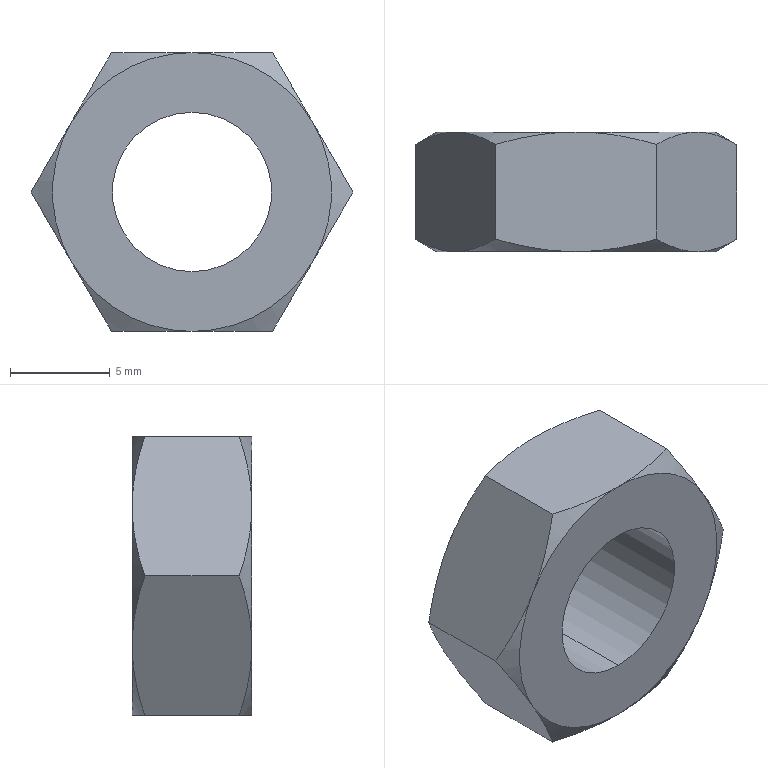Part | 1 solid | 22 faces | box 16.166 x 6 x 14 mm | volume 710.893 mm3 | cone 12 | plane 8 | cylinder 2 | commonest cylinder face diameters 8 x2
STEP:
#1=CARTESIAN_POINT('',(0.,6.,-4.));
#2=VERTEX_POINT('',#1);
#3=CARTESIAN_POINT('',(0.,6.,4.));
#4=VERTEX_POINT('',#3);
#5=CARTESIAN_POINT('',(0.,6.,0.));
#6=DIRECTION('',(0.,1.,0.));
#7=DIRECTION('',(0.,0.,1.));
#8=AXIS2_PLACEMENT_3D('',#5,#6,#7);
#9=CIRCLE('',#8,4.);
#10=EDGE_CURVE('',#2,#4,#9,.T.);
#11=ORIENTED_EDGE('',*,*,#10,.T.);
#12=CARTESIAN_POINT('',(0.,0.,4.));
#13=VERTEX_POINT('',#12);
#14=CARTESIAN_POINT('',(0.,6.,4.));
#15=DIRECTION('',(0.,-1.,0.));
#16=VECTOR('',#15,1000.);
#17=LINE('',#14,#16);
#18=EDGE_CURVE('',#4,#13,#17,.T.);
#19=ORIENTED_EDGE('',*,*,#18,.T.);
#20=CARTESIAN_POINT('',(0.,0.,-4.));
#21=VERTEX_POINT('',#20);
#22=CARTESIAN_POINT('',(0.,0.,0.));
#23=DIRECTION('',(0.,1.,0.));
#24=DIRECTION('',(0.,0.,1.));
#25=AXIS2_PLACEMENT_3D('',#22,#23,#24);
#26=CIRCLE('',#25,4.);
#27=EDGE_CURVE('',#21,#13,#26,.T.);
#28=ORIENTED_EDGE('',*,*,#27,.F.);
#29=CARTESIAN_POINT('',(0.,6.,-4.));
#30=DIRECTION('',(0.,-1.,0.));
#31=VECTOR('',#30,1000.);
#32=LINE('',#29,#31);
#33=EDGE_CURVE('',#2,#21,#32,.T.);
#34=ORIENTED_EDGE('',*,*,#33,.F.);
#35=EDGE_LOOP('',(#11,#19,#28,#34));
#36=FACE_OUTER_BOUND('',#35,.T.);
#37=CARTESIAN_POINT('',(0.,6.,0.));
#38=DIRECTION('',(0.,-1.,0.));
#39=DIRECTION('',(0.,0.,-1.));
#40=AXIS2_PLACEMENT_3D('',#37,#38,#39);
#41=CYLINDRICAL_SURFACE('',#40,4.);
#42=ADVANCED_FACE('',(#36),#41,.F.);
#43=CARTESIAN_POINT('',(8.083,0.6252,0.));
#44=VERTEX_POINT('',#43);
#45=CARTESIAN_POINT('',(6.062,0.,3.5));
#46=VERTEX_POINT('',#45);
#47=CARTESIAN_POINT('',(8.083,0.6252,0.));
#48=CARTESIAN_POINT('',(7.911,0.5258,0.2984));
#49=CARTESIAN_POINT('',(7.742,0.438,0.59));
#50=CARTESIAN_POINT('',(7.493,0.3238,1.021));
#51=CARTESIAN_POINT('',(7.411,0.2886,1.164));
#52=CARTESIAN_POINT('',(7.287,0.2402,1.378));
#53=CARTESIAN_POINT('',(7.226,0.2171,1.484));
#54=CARTESIAN_POINT('',(7.165,0.1957,1.59));
#55=CARTESIAN_POINT('',(7.124,0.1817,1.661));
#56=CARTESIAN_POINT('',(7.104,0.1752,1.695));
#57=CARTESIAN_POINT('',(6.998,0.1408,1.88));
#58=CARTESIAN_POINT('',(6.913,0.1166,2.026));
#59=CARTESIAN_POINT('',(6.786,0.08533,2.246));
#60=CARTESIAN_POINT('',(6.744,0.07574,2.319));
#61=CARTESIAN_POINT('',(6.66,0.05825,2.465));
#62=CARTESIAN_POINT('',(6.619,0.05048,2.536));
#63=CARTESIAN_POINT('',(6.403,0.01442,2.909));
#64=CARTESIAN_POINT('',(6.233,0.,3.203));
#65=CARTESIAN_POINT('',(6.062,0.,3.5));
#66=B_SPLINE_CURVE_WITH_KNOTS('',3,(#47,#48,#49,#50,#51,#52,#53,#54,#55,#56,#57,#58,#59,#60,#61,#62,#63,#64,#65),.UNSPECIFIED.,.F.,.F.,(4,2,2,1,2,2,2,2,2,4),(0.,0.25,0.375,0.4375,0.4687,0.5,0.625,0.6875,0.75,1.),.UNSPECIFIED.);
#67=EDGE_CURVE('',#44,#46,#66,.T.);
#68=ORIENTED_EDGE('',*,*,#67,.F.);
#69=CARTESIAN_POINT('',(8.083,5.375,0.));
#70=VERTEX_POINT('',#69);
#71=CARTESIAN_POINT('',(8.083,6.,0.));
#72=DIRECTION('',(0.,-1.,0.));
#73=VECTOR('',#72,1000.);
#74=LINE('',#71,#73);
#75=EDGE_CURVE('',#70,#44,#74,.T.);
#76=ORIENTED_EDGE('',*,*,#75,.F.);
#77=CARTESIAN_POINT('',(6.062,6.,3.5));
#78=VERTEX_POINT('',#77);
#79=CARTESIAN_POINT('',(6.062,6.,3.5));
#80=CARTESIAN_POINT('',(6.148,6.,3.351));
#81=CARTESIAN_POINT('',(6.233,5.996,3.203));
#82=CARTESIAN_POINT('',(6.362,5.986,2.981));
#83=CARTESIAN_POINT('',(6.405,5.981,2.907));
#84=CARTESIAN_POINT('',(6.49,5.97,2.758));
#85=CARTESIAN_POINT('',(6.534,5.964,2.683));
#86=CARTESIAN_POINT('',(6.661,5.942,2.463));
#87=CARTESIAN_POINT('',(6.745,5.925,2.317));
#88=CARTESIAN_POINT('',(6.872,5.894,2.098));
#89=CARTESIAN_POINT('',(6.935,5.877,1.988));
#90=CARTESIAN_POINT('',(6.999,5.858,1.877));
#91=CARTESIAN_POINT('',(7.042,5.845,1.804));
#92=CARTESIAN_POINT('',(7.064,5.838,1.765));
#93=CARTESIAN_POINT('',(7.411,5.726,1.164));
#94=CARTESIAN_POINT('',(7.739,5.573,0.5959));
#95=CARTESIAN_POINT('',(8.083,5.375,0.));
#96=B_SPLINE_CURVE_WITH_KNOTS('',3,(#79,#80,#81,#82,#83,#84,#85,#86,#87,#88,#89,#90,#91,#92,#93,#94,#95),.UNSPECIFIED.,.F.,.F.,(4,2,2,2,2,1,2,2,4),(0.,0.125,0.1875,0.25,0.375,0.4375,0.4687,0.5,1.),.UNSPECIFIED.);
#97=EDGE_CURVE('',#78,#70,#96,.T.);
#98=ORIENTED_EDGE('',*,*,#97,.F.);
#99=CARTESIAN_POINT('',(4.041,5.375,7.));
#100=VERTEX_POINT('',#99);
#101=CARTESIAN_POINT('',(4.041,5.375,7.));
#102=CARTESIAN_POINT('',(4.214,5.474,6.702));
#103=CARTESIAN_POINT('',(4.382,5.562,6.41));
#104=CARTESIAN_POINT('',(4.631,5.676,5.978));
#105=CARTESIAN_POINT('',(4.714,5.711,5.836));
#106=CARTESIAN_POINT('',(4.837,5.76,5.622));
#107=CARTESIAN_POINT('',(4.898,5.783,5.516));
#108=CARTESIAN_POINT('',(4.96,5.804,5.41));
#109=CARTESIAN_POINT('',(5.001,5.818,5.339));
#110=CARTESIAN_POINT('',(5.02,5.825,5.305));
#111=CARTESIAN_POINT('',(5.127,5.859,5.12));
#112=CARTESIAN_POINT('',(5.211,5.883,4.974));
#113=CARTESIAN_POINT('',(5.338,5.915,4.754));
#114=CARTESIAN_POINT('',(5.38,5.924,4.681));
#115=CARTESIAN_POINT('',(5.465,5.942,4.535));
#116=CARTESIAN_POINT('',(5.506,5.95,4.464));
#117=CARTESIAN_POINT('',(5.721,5.986,4.091));
#118=CARTESIAN_POINT('',(5.891,6.,3.797));
#119=CARTESIAN_POINT('',(6.062,6.,3.5));
#120=B_SPLINE_CURVE_WITH_KNOTS('',3,(#101,#102,#103,#104,#105,#106,#107,#108,#109,#110,#111,#112,#113,#114,#115,#116,#117,#118,#119),.UNSPECIFIED.,.F.,.F.,(4,2,2,1,2,2,2,2,2,4),(0.,0.25,0.375,0.4375,0.4688,0.5,0.625,0.6875,0.75,1.),.UNSPECIFIED.);
#121=EDGE_CURVE('',#100,#78,#120,.T.);
#122=ORIENTED_EDGE('',*,*,#121,.F.);
#123=CARTESIAN_POINT('',(4.041,0.6252,7.));
#124=VERTEX_POINT('',#123);
#125=CARTESIAN_POINT('',(4.041,6.,7.));
#126=DIRECTION('',(0.,-1.,0.));
#127=VECTOR('',#126,1000.);
#128=LINE('',#125,#127);
#129=EDGE_CURVE('',#100,#124,#128,.T.);
#130=ORIENTED_EDGE('',*,*,#129,.T.);
#131=CARTESIAN_POINT('',(6.062,0.,3.5));
#132=CARTESIAN_POINT('',(5.976,0.,3.649));
#133=CARTESIAN_POINT('',(5.891,0.003614,3.797));
#134=CARTESIAN_POINT('',(5.763,0.01446,4.019));
#135=CARTESIAN_POINT('',(5.72,0.01898,4.093));
#136=CARTESIAN_POINT('',(5.634,0.02982,4.242));
#137=CARTESIAN_POINT('',(5.59,0.03629,4.317));
#138=CARTESIAN_POINT('',(5.464,0.05753,4.537));
#139=CARTESIAN_POINT('',(5.379,0.07506,4.683));
#140=CARTESIAN_POINT('',(5.253,0.1064,4.902));
#141=CARTESIAN_POINT('',(5.189,0.1234,5.012));
#142=CARTESIAN_POINT('',(5.125,0.1422,5.123));
#143=CARTESIAN_POINT('',(5.083,0.1552,5.196));
#144=CARTESIAN_POINT('',(5.061,0.1622,5.235));
#145=CARTESIAN_POINT('',(4.714,0.2744,5.836));
#146=CARTESIAN_POINT('',(4.386,0.4266,6.404));
#147=CARTESIAN_POINT('',(4.041,0.6252,7.));
#148=B_SPLINE_CURVE_WITH_KNOTS('',3,(#131,#132,#133,#134,#135,#136,#137,#138,#139,#140,#141,#142,#143,#144,#145,#146,#147),.UNSPECIFIED.,.F.,.F.,(4,2,2,2,2,1,2,2,4),(0.,0.125,0.1875,0.25,0.375,0.4375,0.4687,0.5,1.),.UNSPECIFIED.);
#149=EDGE_CURVE('',#46,#124,#148,.T.);
#150=ORIENTED_EDGE('',*,*,#149,.F.);
#151=EDGE_LOOP('',(#68,#76,#98,#122,#130,#150));
#152=FACE_OUTER_BOUND('',#151,.T.);
#153=CARTESIAN_POINT('',(4.041,6.,7.));
#154=DIRECTION('',(-0.866,0.,-0.5));
#155=DIRECTION('',(-0.5,0.,0.866));
#156=AXIS2_PLACEMENT_3D('',#153,#154,#155);
#157=PLANE('',#156);
#158=ADVANCED_FACE('',(#152),#157,.F.);
#159=CARTESIAN_POINT('',(4.041,0.6252,-7.));
#160=VERTEX_POINT('',#159);
#161=CARTESIAN_POINT('',(6.062,0.,-3.5));
#162=VERTEX_POINT('',#161);
#163=CARTESIAN_POINT('',(4.041,0.6252,-7.));
#164=CARTESIAN_POINT('',(4.214,0.5258,-6.702));
#165=CARTESIAN_POINT('',(4.382,0.438,-6.41));
#166=CARTESIAN_POINT('',(4.631,0.3238,-5.978));
#167=CARTESIAN_POINT('',(4.714,0.2886,-5.836));
#168=CARTESIAN_POINT('',(4.837,0.2402,-5.622));
#169=CARTESIAN_POINT('',(4.898,0.2171,-5.516));
#170=CARTESIAN_POINT('',(4.96,0.1957,-5.41));
#171=CARTESIAN_POINT('',(5.001,0.1817,-5.339));
#172=CARTESIAN_POINT('',(5.02,0.1752,-5.305));
#173=CARTESIAN_POINT('',(5.127,0.1408,-5.12));
#174=CARTESIAN_POINT('',(5.211,0.1166,-4.974));
#175=CARTESIAN_POINT('',(5.338,0.08533,-4.754));
#176=CARTESIAN_POINT('',(5.38,0.07574,-4.681));
#177=CARTESIAN_POINT('',(5.465,0.05825,-4.535));
#178=CARTESIAN_POINT('',(5.506,0.05048,-4.464));
#179=CARTESIAN_POINT('',(5.721,0.01442,-4.091));
#180=CARTESIAN_POINT('',(5.891,0.,-3.797));
#181=CARTESIAN_POINT('',(6.062,0.,-3.5));
#182=B_SPLINE_CURVE_WITH_KNOTS('',3,(#163,#164,#165,#166,#167,#168,#169,#170,#171,#172,#173,#174,#175,#176,#177,#178,#179,#180,#181),.UNSPECIFIED.,.F.,.F.,(4,2,2,1,2,2,2,2,2,4),(0.,0.25,0.375,0.4375,0.4687,0.5,0.625,0.6875,0.75,1.),.UNSPECIFIED.);
#183=EDGE_CURVE('',#160,#162,#182,.T.);
#184=ORIENTED_EDGE('',*,*,#183,.F.);
#185=CARTESIAN_POINT('',(4.041,5.375,-7.));
#186=VERTEX_POINT('',#185);
#187=CARTESIAN_POINT('',(4.041,6.,-7.));
#188=DIRECTION('',(0.,-1.,0.));
#189=VECTOR('',#188,1000.);
#190=LINE('',#187,#189);
#191=EDGE_CURVE('',#186,#160,#190,.T.);
#192=ORIENTED_EDGE('',*,*,#191,.F.);
#193=CARTESIAN_POINT('',(6.062,6.,-3.5));
#194=VERTEX_POINT('',#193);
#195=CARTESIAN_POINT('',(6.062,6.,-3.5));
#196=CARTESIAN_POINT('',(5.976,6.,-3.649));
#197=CARTESIAN_POINT('',(5.891,5.996,-3.797));
#198=CARTESIAN_POINT('',(5.763,5.986,-4.019));
#199=CARTESIAN_POINT('',(5.72,5.981,-4.093));
#200=CARTESIAN_POINT('',(5.634,5.97,-4.242));
#201=CARTESIAN_POINT('',(5.59,5.964,-4.317));
#202=CARTESIAN_POINT('',(5.464,5.942,-4.537));
#203=CARTESIAN_POINT('',(5.379,5.925,-4.683));
#204=CARTESIAN_POINT('',(5.253,5.894,-4.902));
#205=CARTESIAN_POINT('',(5.189,5.877,-5.012));
#206=CARTESIAN_POINT('',(5.125,5.858,-5.123));
#207=CARTESIAN_POINT('',(5.083,5.845,-5.196));
#208=CARTESIAN_POINT('',(5.061,5.838,-5.235));
#209=CARTESIAN_POINT('',(4.714,5.726,-5.836));
#210=CARTESIAN_POINT('',(4.386,5.573,-6.404));
#211=CARTESIAN_POINT('',(4.041,5.375,-7.));
#212=B_SPLINE_CURVE_WITH_KNOTS('',3,(#195,#196,#197,#198,#199,#200,#201,#202,#203,#204,#205,#206,#207,#208,#209,#210,#211),.UNSPECIFIED.,.F.,.F.,(4,2,2,2,2,1,2,2,4),(0.,0.125,0.1875,0.25,0.375,0.4375,0.4687,0.5,1.),.UNSPECIFIED.);
#213=EDGE_CURVE('',#194,#186,#212,.T.);
#214=ORIENTED_EDGE('',*,*,#213,.F.);
#215=CARTESIAN_POINT('',(8.083,5.375,0.));
#216=CARTESIAN_POINT('',(7.911,5.474,-0.2984));
#217=CARTESIAN_POINT('',(7.742,5.562,-0.59));
#218=CARTESIAN_POINT('',(7.493,5.676,-1.021));
#219=CARTESIAN_POINT('',(7.411,5.711,-1.164));
#220=CARTESIAN_POINT('',(7.287,5.76,-1.378));
#221=CARTESIAN_POINT('',(7.226,5.783,-1.484));
#222=CARTESIAN_POINT('',(7.165,5.804,-1.59));
#223=CARTESIAN_POINT('',(7.124,5.818,-1.661));
#224=CARTESIAN_POINT('',(7.104,5.825,-1.695));
#225=CARTESIAN_POINT('',(6.998,5.859,-1.88));
#226=CARTESIAN_POINT('',(6.913,5.883,-2.026));
#227=CARTESIAN_POINT('',(6.786,5.915,-2.246));
#228=CARTESIAN_POINT('',(6.744,5.924,-2.319));
#229=CARTESIAN_POINT('',(6.66,5.942,-2.465));
#230=CARTESIAN_POINT('',(6.619,5.95,-2.536));
#231=CARTESIAN_POINT('',(6.403,5.986,-2.909));
#232=CARTESIAN_POINT('',(6.233,6.,-3.203));
#233=CARTESIAN_POINT('',(6.062,6.,-3.5));
#234=B_SPLINE_CURVE_WITH_KNOTS('',3,(#215,#216,#217,#218,#219,#220,#221,#222,#223,#224,#225,#226,#227,#228,#229,#230,#231,#232,#233),.UNSPECIFIED.,.F.,.F.,(4,2,2,1,2,2,2,2,2,4),(0.,0.25,0.375,0.4375,0.4688,0.5,0.625,0.6875,0.75,1.),.UNSPECIFIED.);
#235=EDGE_CURVE('',#70,#194,#234,.T.);
#236=ORIENTED_EDGE('',*,*,#235,.F.);
#237=ORIENTED_EDGE('',*,*,#75,.T.);
#238=CARTESIAN_POINT('',(6.062,0.,-3.5));
#239=CARTESIAN_POINT('',(6.148,0.,-3.351));
#240=CARTESIAN_POINT('',(6.233,0.003614,-3.203));
#241=CARTESIAN_POINT('',(6.362,0.01446,-2.981));
#242=CARTESIAN_POINT('',(6.405,0.01898,-2.907));
#243=CARTESIAN_POINT('',(6.49,0.02982,-2.758));
#244=CARTESIAN_POINT('',(6.534,0.03629,-2.683));
#245=CARTESIAN_POINT('',(6.661,0.05753,-2.463));
#246=CARTESIAN_POINT('',(6.745,0.07506,-2.317));
#247=CARTESIAN_POINT('',(6.872,0.1064,-2.098));
#248=CARTESIAN_POINT('',(6.935,0.1234,-1.988));
#249=CARTESIAN_POINT('',(6.999,0.1422,-1.877));
#250=CARTESIAN_POINT('',(7.042,0.1552,-1.804));
#251=CARTESIAN_POINT('',(7.064,0.1622,-1.765));
#252=CARTESIAN_POINT('',(7.411,0.2744,-1.164));
#253=CARTESIAN_POINT('',(7.739,0.4266,-0.5959));
#254=CARTESIAN_POINT('',(8.083,0.6252,0.));
#255=B_SPLINE_CURVE_WITH_KNOTS('',3,(#238,#239,#240,#241,#242,#243,#244,#245,#246,#247,#248,#249,#250,#251,#252,#253,#254),.UNSPECIFIED.,.F.,.F.,(4,2,2,2,2,1,2,2,4),(0.,0.125,0.1875,0.25,0.375,0.4375,0.4688,0.5,1.),.UNSPECIFIED.);
#256=EDGE_CURVE('',#162,#44,#255,.T.);
#257=ORIENTED_EDGE('',*,*,#256,.F.);
#258=EDGE_LOOP('',(#184,#192,#214,#236,#237,#257));
#259=FACE_OUTER_BOUND('',#258,.T.);
#260=CARTESIAN_POINT('',(8.083,6.,0.));
#261=DIRECTION('',(-0.866,0.,0.5));
#262=DIRECTION('',(0.,1.,0.));
#263=AXIS2_PLACEMENT_3D('',#260,#261,#262);
#264=PLANE('',#263);
#265=ADVANCED_FACE('',(#259),#264,.F.);
#266=CARTESIAN_POINT('',(-4.041,0.6252,-7.));
#267=VERTEX_POINT('',#266);
#268=CARTESIAN_POINT('',(0.,0.,-7.));
#269=VERTEX_POINT('',#268);
#270=CARTESIAN_POINT('',(-4.041,0.6252,-7.));
#271=CARTESIAN_POINT('',(-3.696,0.5255,-7.));
#272=CARTESIAN_POINT('',(-3.358,0.4375,-7.));
#273=CARTESIAN_POINT('',(-2.859,0.3231,-7.));
#274=CARTESIAN_POINT('',(-2.694,0.2879,-7.));
#275=CARTESIAN_POINT('',(-2.447,0.2395,-7.));
#276=CARTESIAN_POINT('',(-2.323,0.2164,-7.));
#277=CARTESIAN_POINT('',(-2.2,0.1949,-7.));
#278=CARTESIAN_POINT('',(-2.118,0.1809,-7.));
#279=CARTESIAN_POINT('',(-2.079,0.1744,-7.));
#280=CARTESIAN_POINT('',(-1.866,0.1401,-7.));
#281=CARTESIAN_POINT('',(-1.697,0.1159,-7.));
#282=CARTESIAN_POINT('',(-1.443,0.08477,-7.));
#283=CARTESIAN_POINT('',(-1.359,0.07522,-7.));
#284=CARTESIAN_POINT('',(-1.191,0.05779,-7.));
#285=CARTESIAN_POINT('',(-1.108,0.05002,-7.));
#286=CARTESIAN_POINT('',(-0.6791,0.01429,-7.));
#287=CARTESIAN_POINT('',(-0.3408,0.,-7.));
#288=CARTESIAN_POINT('',(0.,0.,-7.));
#289=B_SPLINE_CURVE_WITH_KNOTS('',3,(#270,#271,#272,#273,#274,#275,#276,#277,#278,#279,#280,#281,#282,#283,#284,#285,#286,#287,#288),.UNSPECIFIED.,.F.,.F.,(4,2,2,1,2,2,2,2,2,4),(0.,0.25,0.375,0.4375,0.4687,0.5,0.625,0.6875,0.75,1.),.UNSPECIFIED.);
#290=EDGE_CURVE('',#267,#269,#289,.T.);
#291=ORIENTED_EDGE('',*,*,#290,.F.);
#292=CARTESIAN_POINT('',(-4.041,5.375,-7.));
#293=VERTEX_POINT('',#292);
#294=CARTESIAN_POINT('',(-4.041,6.,-7.));
#295=DIRECTION('',(0.,-1.,0.));
#296=VECTOR('',#295,1000.);
#297=LINE('',#294,#296);
#298=EDGE_CURVE('',#293,#267,#297,.T.);
#299=ORIENTED_EDGE('',*,*,#298,.F.);
#300=CARTESIAN_POINT('',(0.,6.,-7.));
#301=VERTEX_POINT('',#300);
#302=CARTESIAN_POINT('',(0.,6.,-7.));
#303=CARTESIAN_POINT('',(-0.1704,6.,-7.));
#304=CARTESIAN_POINT('',(-0.3402,5.996,-7.));
#305=CARTESIAN_POINT('',(-0.5952,5.986,-7.));
#306=CARTESIAN_POINT('',(-0.6803,5.981,-7.));
#307=CARTESIAN_POINT('',(-0.8507,5.971,-7.));
#308=CARTESIAN_POINT('',(-0.9375,5.964,-7.));
#309=CARTESIAN_POINT('',(-1.191,5.943,-7.));
#310=CARTESIAN_POINT('',(-1.359,5.926,-7.));
#311=CARTESIAN_POINT('',(-1.612,5.894,-7.));
#312=CARTESIAN_POINT('',(-1.739,5.878,-7.));
#313=CARTESIAN_POINT('',(-1.866,5.859,-7.));
#314=CARTESIAN_POINT('',(-1.951,5.846,-7.));
#315=CARTESIAN_POINT('',(-1.995,5.839,-7.));
#316=CARTESIAN_POINT('',(-2.692,5.727,-7.));
#317=CARTESIAN_POINT('',(-3.351,5.574,-7.));
#318=CARTESIAN_POINT('',(-4.041,5.375,-7.));
#319=B_SPLINE_CURVE_WITH_KNOTS('',3,(#302,#303,#304,#305,#306,#307,#308,#309,#310,#311,#312,#313,#314,#315,#316,#317,#318),.UNSPECIFIED.,.F.,.F.,(4,2,2,2,2,1,2,2,4),(0.,0.125,0.1875,0.25,0.375,0.4375,0.4687,0.5,1.),.UNSPECIFIED.);
#320=EDGE_CURVE('',#301,#293,#319,.T.);
#321=ORIENTED_EDGE('',*,*,#320,.F.);
#322=CARTESIAN_POINT('',(4.041,5.375,-7.));
#323=CARTESIAN_POINT('',(3.699,5.474,-7.));
#324=CARTESIAN_POINT('',(3.364,5.561,-7.));
#325=CARTESIAN_POINT('',(2.868,5.675,-7.));
#326=CARTESIAN_POINT('',(2.704,5.71,-7.));
#327=CARTESIAN_POINT('',(2.459,5.758,-7.));
#328=CARTESIAN_POINT('',(2.336,5.781,-7.));
#329=CARTESIAN_POINT('',(2.214,5.803,-7.));
#330=CARTESIAN_POINT('',(2.133,5.817,-7.));
#331=CARTESIAN_POINT('',(2.094,5.823,-7.));
#332=CARTESIAN_POINT('',(1.88,5.858,-7.));
#333=CARTESIAN_POINT('',(1.71,5.882,-7.));
#334=CARTESIAN_POINT('',(1.455,5.914,-7.));
#335=CARTESIAN_POINT('',(1.37,5.924,-7.));
#336=CARTESIAN_POINT('',(1.2,5.941,-7.));
#337=CARTESIAN_POINT('',(1.116,5.949,-7.));
#338=CARTESIAN_POINT('',(0.6836,5.985,-7.));
#339=CARTESIAN_POINT('',(0.3428,6.,-7.));
#340=CARTESIAN_POINT('',(0.,6.,-7.));
#341=B_SPLINE_CURVE_WITH_KNOTS('',3,(#322,#323,#324,#325,#326,#327,#328,#329,#330,#331,#332,#333,#334,#335,#336,#337,#338,#339,#340),.UNSPECIFIED.,.F.,.F.,(4,2,2,1,2,2,2,2,2,4),(0.,0.25,0.375,0.4375,0.4688,0.5,0.625,0.6875,0.75,1.),.UNSPECIFIED.);
#342=EDGE_CURVE('',#186,#301,#341,.T.);
#343=ORIENTED_EDGE('',*,*,#342,.F.);
#344=ORIENTED_EDGE('',*,*,#191,.T.);
#345=CARTESIAN_POINT('',(0.,0.,-7.));
#346=CARTESIAN_POINT('',(0.1714,0.,-7.));
#347=CARTESIAN_POINT('',(0.3423,0.003632,-7.));
#348=CARTESIAN_POINT('',(0.5992,0.01453,-7.));
#349=CARTESIAN_POINT('',(0.685,0.01907,-7.));
#350=CARTESIAN_POINT('',(0.8569,0.02997,-7.));
#351=CARTESIAN_POINT('',(0.9444,0.03644,-7.));
#352=CARTESIAN_POINT('',(1.2,0.05789,-7.));
#353=CARTESIAN_POINT('',(1.37,0.07557,-7.));
#354=CARTESIAN_POINT('',(1.625,0.1072,-7.));
#355=CARTESIAN_POINT('',(1.752,0.1242,-7.));
#356=CARTESIAN_POINT('',(1.88,0.1432,-7.));
#357=CARTESIAN_POINT('',(1.966,0.1563,-7.));
#358=CARTESIAN_POINT('',(2.011,0.1634,-7.));
#359=CARTESIAN_POINT('',(2.702,0.2756,-7.));
#360=CARTESIAN_POINT('',(3.356,0.4273,-7.));
#361=CARTESIAN_POINT('',(4.041,0.6252,-7.));
#362=B_SPLINE_CURVE_WITH_KNOTS('',3,(#345,#346,#347,#348,#349,#350,#351,#352,#353,#354,#355,#356,#357,#358,#359,#360,#361),.UNSPECIFIED.,.F.,.F.,(4,2,2,2,2,1,2,2,4),(0.,0.125,0.1875,0.25,0.375,0.4375,0.4687,0.5,1.),.UNSPECIFIED.);
#363=EDGE_CURVE('',#269,#160,#362,.T.);
#364=ORIENTED_EDGE('',*,*,#363,.F.);
#365=EDGE_LOOP('',(#291,#299,#321,#343,#344,#364));
#366=FACE_OUTER_BOUND('',#365,.T.);
#367=CARTESIAN_POINT('',(4.041,6.,-7.));
#368=DIRECTION('',(0.,0.,1.));
#369=DIRECTION('',(1.,0.,0.));
#370=AXIS2_PLACEMENT_3D('',#367,#368,#369);
#371=PLANE('',#370);
#372=ADVANCED_FACE('',(#366),#371,.F.);
#373=CARTESIAN_POINT('',(-8.083,0.6252,0.));
#374=VERTEX_POINT('',#373);
#375=CARTESIAN_POINT('',(-6.062,0.,-3.5));
#376=VERTEX_POINT('',#375);
#377=CARTESIAN_POINT('',(-8.083,0.6252,0.));
#378=CARTESIAN_POINT('',(-7.911,0.5258,-0.2984));
#379=CARTESIAN_POINT('',(-7.742,0.438,-0.59));
#380=CARTESIAN_POINT('',(-7.493,0.3238,-1.021));
#381=CARTESIAN_POINT('',(-7.411,0.2886,-1.164));
#382=CARTESIAN_POINT('',(-7.287,0.2402,-1.378));
#383=CARTESIAN_POINT('',(-7.226,0.2171,-1.484));
#384=CARTESIAN_POINT('',(-7.165,0.1957,-1.59));
#385=CARTESIAN_POINT('',(-7.124,0.1817,-1.661));
#386=CARTESIAN_POINT('',(-7.104,0.1752,-1.695));
#387=CARTESIAN_POINT('',(-6.998,0.1408,-1.88));
#388=CARTESIAN_POINT('',(-6.913,0.1166,-2.026));
#389=CARTESIAN_POINT('',(-6.786,0.08533,-2.246));
#390=CARTESIAN_POINT('',(-6.744,0.07574,-2.319));
#391=CARTESIAN_POINT('',(-6.66,0.05825,-2.465));
#392=CARTESIAN_POINT('',(-6.619,0.05048,-2.536));
#393=CARTESIAN_POINT('',(-6.403,0.01442,-2.909));
#394=CARTESIAN_POINT('',(-6.233,0.,-3.203));
#395=CARTESIAN_POINT('',(-6.062,0.,-3.5));
#396=B_SPLINE_CURVE_WITH_KNOTS('',3,(#377,#378,#379,#380,#381,#382,#383,#384,#385,#386,#387,#388,#389,#390,#391,#392,#393,#394,#395),.UNSPECIFIED.,.F.,.F.,(4,2,2,1,2,2,2,2,2,4),(0.,0.25,0.375,0.4375,0.4687,0.5,0.625,0.6875,0.75,1.),.UNSPECIFIED.);
#397=EDGE_CURVE('',#374,#376,#396,.T.);
#398=ORIENTED_EDGE('',*,*,#397,.F.);
#399=CARTESIAN_POINT('',(-8.083,5.375,0.));
#400=VERTEX_POINT('',#399);
#401=CARTESIAN_POINT('',(-8.083,6.,0.));
#402=DIRECTION('',(0.,-1.,0.));
#403=VECTOR('',#402,1000.);
#404=LINE('',#401,#403);
#405=EDGE_CURVE('',#400,#374,#404,.T.);
#406=ORIENTED_EDGE('',*,*,#405,.F.);
#407=CARTESIAN_POINT('',(-6.062,6.,-3.5));
#408=VERTEX_POINT('',#407);
#409=CARTESIAN_POINT('',(-6.062,6.,-3.5));
#410=CARTESIAN_POINT('',(-6.148,6.,-3.351));
#411=CARTESIAN_POINT('',(-6.233,5.996,-3.203));
#412=CARTESIAN_POINT('',(-6.362,5.986,-2.981));
#413=CARTESIAN_POINT('',(-6.405,5.981,-2.907));
#414=CARTESIAN_POINT('',(-6.49,5.97,-2.758));
#415=CARTESIAN_POINT('',(-6.534,5.964,-2.683));
#416=CARTESIAN_POINT('',(-6.661,5.942,-2.463));
#417=CARTESIAN_POINT('',(-6.745,5.925,-2.317));
#418=CARTESIAN_POINT('',(-6.872,5.894,-2.098));
#419=CARTESIAN_POINT('',(-6.935,5.877,-1.988));
#420=CARTESIAN_POINT('',(-6.999,5.858,-1.877));
#421=CARTESIAN_POINT('',(-7.042,5.845,-1.804));
#422=CARTESIAN_POINT('',(-7.064,5.838,-1.765));
#423=CARTESIAN_POINT('',(-7.411,5.726,-1.164));
#424=CARTESIAN_POINT('',(-7.739,5.573,-0.5959));
#425=CARTESIAN_POINT('',(-8.083,5.375,0.));
#426=B_SPLINE_CURVE_WITH_KNOTS('',3,(#409,#410,#411,#412,#413,#414,#415,#416,#417,#418,#419,#420,#421,#422,#423,#424,#425),.UNSPECIFIED.,.F.,.F.,(4,2,2,2,2,1,2,2,4),(0.,0.125,0.1875,0.25,0.375,0.4375,0.4687,0.5,1.),.UNSPECIFIED.);
#427=EDGE_CURVE('',#408,#400,#426,.T.);
#428=ORIENTED_EDGE('',*,*,#427,.F.);
#429=CARTESIAN_POINT('',(-4.041,5.375,-7.));
#430=CARTESIAN_POINT('',(-4.214,5.474,-6.702));
#431=CARTESIAN_POINT('',(-4.382,5.562,-6.41));
#432=CARTESIAN_POINT('',(-4.631,5.676,-5.978));
#433=CARTESIAN_POINT('',(-4.714,5.711,-5.836));
#434=CARTESIAN_POINT('',(-4.837,5.76,-5.622));
#435=CARTESIAN_POINT('',(-4.898,5.783,-5.516));
#436=CARTESIAN_POINT('',(-4.96,5.804,-5.41));
#437=CARTESIAN_POINT('',(-5.001,5.818,-5.339));
#438=CARTESIAN_POINT('',(-5.02,5.825,-5.305));
#439=CARTESIAN_POINT('',(-5.127,5.859,-5.12));
#440=CARTESIAN_POINT('',(-5.211,5.883,-4.974));
#441=CARTESIAN_POINT('',(-5.338,5.915,-4.754));
#442=CARTESIAN_POINT('',(-5.38,5.924,-4.681));
#443=CARTESIAN_POINT('',(-5.465,5.942,-4.535));
#444=CARTESIAN_POINT('',(-5.506,5.95,-4.464));
#445=CARTESIAN_POINT('',(-5.721,5.986,-4.091));
#446=CARTESIAN_POINT('',(-5.891,6.,-3.797));
#447=CARTESIAN_POINT('',(-6.062,6.,-3.5));
#448=B_SPLINE_CURVE_WITH_KNOTS('',3,(#429,#430,#431,#432,#433,#434,#435,#436,#437,#438,#439,#440,#441,#442,#443,#444,#445,#446,#447),.UNSPECIFIED.,.F.,.F.,(4,2,2,1,2,2,2,2,2,4),(0.,0.25,0.375,0.4375,0.4688,0.5,0.625,0.6875,0.75,1.),.UNSPECIFIED.);
#449=EDGE_CURVE('',#293,#408,#448,.T.);
#450=ORIENTED_EDGE('',*,*,#449,.F.);
#451=ORIENTED_EDGE('',*,*,#298,.T.);
#452=CARTESIAN_POINT('',(-6.062,0.,-3.5));
#453=CARTESIAN_POINT('',(-5.976,0.,-3.649));
#454=CARTESIAN_POINT('',(-5.891,0.003614,-3.797));
#455=CARTESIAN_POINT('',(-5.763,0.01446,-4.019));
#456=CARTESIAN_POINT('',(-5.72,0.01898,-4.093));
#457=CARTESIAN_POINT('',(-5.634,0.02982,-4.242));
#458=CARTESIAN_POINT('',(-5.59,0.03629,-4.317));
#459=CARTESIAN_POINT('',(-5.464,0.05753,-4.537));
#460=CARTESIAN_POINT('',(-5.379,0.07506,-4.683));
#461=CARTESIAN_POINT('',(-5.253,0.1064,-4.902));
#462=CARTESIAN_POINT('',(-5.189,0.1234,-5.012));
#463=CARTESIAN_POINT('',(-5.125,0.1422,-5.123));
#464=CARTESIAN_POINT('',(-5.083,0.1552,-5.196));
#465=CARTESIAN_POINT('',(-5.061,0.1622,-5.235));
#466=CARTESIAN_POINT('',(-4.714,0.2744,-5.836));
#467=CARTESIAN_POINT('',(-4.386,0.4266,-6.404));
#468=CARTESIAN_POINT('',(-4.041,0.6252,-7.));
#469=B_SPLINE_CURVE_WITH_KNOTS('',3,(#452,#453,#454,#455,#456,#457,#458,#459,#460,#461,#462,#463,#464,#465,#466,#467,#468),.UNSPECIFIED.,.F.,.F.,(4,2,2,2,2,1,2,2,4),(0.,0.125,0.1875,0.25,0.375,0.4375,0.4687,0.5,1.),.UNSPECIFIED.);
#470=EDGE_CURVE('',#376,#267,#469,.T.);
#471=ORIENTED_EDGE('',*,*,#470,.F.);
#472=EDGE_LOOP('',(#398,#406,#428,#450,#451,#471));
#473=FACE_OUTER_BOUND('',#472,.T.);
#474=CARTESIAN_POINT('',(-4.041,6.,-7.));
#475=DIRECTION('',(0.866,0.,0.5));
#476=DIRECTION('',(0.,-1.,0.));
#477=AXIS2_PLACEMENT_3D('',#474,#475,#476);
#478=PLANE('',#477);
#479=ADVANCED_FACE('',(#473),#478,.F.);
#480=CARTESIAN_POINT('',(-4.041,0.6252,7.));
#481=VERTEX_POINT('',#480);
#482=CARTESIAN_POINT('',(-6.062,0.,3.5));
#483=VERTEX_POINT('',#482);
#484=CARTESIAN_POINT('',(-4.041,0.6252,7.));
#485=CARTESIAN_POINT('',(-4.214,0.5258,6.702));
#486=CARTESIAN_POINT('',(-4.382,0.438,6.41));
#487=CARTESIAN_POINT('',(-4.631,0.3238,5.978));
#488=CARTESIAN_POINT('',(-4.714,0.2886,5.836));
#489=CARTESIAN_POINT('',(-4.837,0.2402,5.622));
#490=CARTESIAN_POINT('',(-4.898,0.2171,5.516));
#491=CARTESIAN_POINT('',(-4.96,0.1957,5.41));
#492=CARTESIAN_POINT('',(-5.001,0.1817,5.339));
#493=CARTESIAN_POINT('',(-5.02,0.1752,5.305));
#494=CARTESIAN_POINT('',(-5.127,0.1408,5.12));
#495=CARTESIAN_POINT('',(-5.211,0.1166,4.974));
#496=CARTESIAN_POINT('',(-5.338,0.08533,4.754));
#497=CARTESIAN_POINT('',(-5.38,0.07574,4.681));
#498=CARTESIAN_POINT('',(-5.465,0.05825,4.535));
#499=CARTESIAN_POINT('',(-5.506,0.05048,4.464));
#500=CARTESIAN_POINT('',(-5.721,0.01442,4.091));
#501=CARTESIAN_POINT('',(-5.891,0.,3.797));
#502=CARTESIAN_POINT('',(-6.062,0.,3.5));
#503=B_SPLINE_CURVE_WITH_KNOTS('',3,(#484,#485,#486,#487,#488,#489,#490,#491,#492,#493,#494,#495,#496,#497,#498,#499,#500,#501,#502),.UNSPECIFIED.,.F.,.F.,(4,2,2,1,2,2,2,2,2,4),(0.,0.25,0.375,0.4375,0.4687,0.5,0.625,0.6875,0.75,1.),.UNSPECIFIED.);
#504=EDGE_CURVE('',#481,#483,#503,.T.);
#505=ORIENTED_EDGE('',*,*,#504,.F.);
#506=CARTESIAN_POINT('',(-4.041,5.375,7.));
#507=VERTEX_POINT('',#506);
#508=CARTESIAN_POINT('',(-4.041,6.,7.));
#509=DIRECTION('',(0.,-1.,0.));
#510=VECTOR('',#509,1000.);
#511=LINE('',#508,#510);
#512=EDGE_CURVE('',#507,#481,#511,.T.);
#513=ORIENTED_EDGE('',*,*,#512,.F.);
#514=CARTESIAN_POINT('',(-6.062,6.,3.5));
#515=VERTEX_POINT('',#514);
#516=CARTESIAN_POINT('',(-6.062,6.,3.5));
#517=CARTESIAN_POINT('',(-5.976,6.,3.649));
#518=CARTESIAN_POINT('',(-5.891,5.996,3.797));
#519=CARTESIAN_POINT('',(-5.763,5.986,4.019));
#520=CARTESIAN_POINT('',(-5.72,5.981,4.093));
#521=CARTESIAN_POINT('',(-5.634,5.97,4.242));
#522=CARTESIAN_POINT('',(-5.59,5.964,4.317));
#523=CARTESIAN_POINT('',(-5.464,5.942,4.537));
#524=CARTESIAN_POINT('',(-5.379,5.925,4.683));
#525=CARTESIAN_POINT('',(-5.253,5.894,4.902));
#526=CARTESIAN_POINT('',(-5.189,5.877,5.012));
#527=CARTESIAN_POINT('',(-5.125,5.858,5.123));
#528=CARTESIAN_POINT('',(-5.083,5.845,5.196));
#529=CARTESIAN_POINT('',(-5.061,5.838,5.235));
#530=CARTESIAN_POINT('',(-4.714,5.726,5.836));
#531=CARTESIAN_POINT('',(-4.386,5.573,6.404));
#532=CARTESIAN_POINT('',(-4.041,5.375,7.));
#533=B_SPLINE_CURVE_WITH_KNOTS('',3,(#516,#517,#518,#519,#520,#521,#522,#523,#524,#525,#526,#527,#528,#529,#530,#531,#532),.UNSPECIFIED.,.F.,.F.,(4,2,2,2,2,1,2,2,4),(0.,0.125,0.1875,0.25,0.375,0.4375,0.4687,0.5,1.),.UNSPECIFIED.);
#534=EDGE_CURVE('',#515,#507,#533,.T.);
#535=ORIENTED_EDGE('',*,*,#534,.F.);
#536=CARTESIAN_POINT('',(-8.083,5.375,0.));
#537=CARTESIAN_POINT('',(-7.911,5.474,0.2984));
#538=CARTESIAN_POINT('',(-7.742,5.562,0.59));
#539=CARTESIAN_POINT('',(-7.493,5.676,1.021));
#540=CARTESIAN_POINT('',(-7.411,5.711,1.164));
#541=CARTESIAN_POINT('',(-7.287,5.76,1.378));
#542=CARTESIAN_POINT('',(-7.226,5.783,1.484));
#543=CARTESIAN_POINT('',(-7.165,5.804,1.59));
#544=CARTESIAN_POINT('',(-7.124,5.818,1.661));
#545=CARTESIAN_POINT('',(-7.104,5.825,1.695));
#546=CARTESIAN_POINT('',(-6.998,5.859,1.88));
#547=CARTESIAN_POINT('',(-6.913,5.883,2.026));
#548=CARTESIAN_POINT('',(-6.786,5.915,2.246));
#549=CARTESIAN_POINT('',(-6.744,5.924,2.319));
#550=CARTESIAN_POINT('',(-6.66,5.942,2.465));
#551=CARTESIAN_POINT('',(-6.619,5.95,2.536));
#552=CARTESIAN_POINT('',(-6.403,5.986,2.909));
#553=CARTESIAN_POINT('',(-6.233,6.,3.203));
#554=CARTESIAN_POINT('',(-6.062,6.,3.5));
#555=B_SPLINE_CURVE_WITH_KNOTS('',3,(#536,#537,#538,#539,#540,#541,#542,#543,#544,#545,#546,#547,#548,#549,#550,#551,#552,#553,#554),.UNSPECIFIED.,.F.,.F.,(4,2,2,1,2,2,2,2,2,4),(0.,0.25,0.375,0.4375,0.4688,0.5,0.625,0.6875,0.75,1.),.UNSPECIFIED.);
#556=EDGE_CURVE('',#400,#515,#555,.T.);
#557=ORIENTED_EDGE('',*,*,#556,.F.);
#558=ORIENTED_EDGE('',*,*,#405,.T.);
#559=CARTESIAN_POINT('',(-6.062,0.,3.5));
#560=CARTESIAN_POINT('',(-6.148,0.,3.351));
#561=CARTESIAN_POINT('',(-6.233,0.003614,3.203));
#562=CARTESIAN_POINT('',(-6.362,0.01446,2.981));
#563=CARTESIAN_POINT('',(-6.405,0.01898,2.907));
#564=CARTESIAN_POINT('',(-6.49,0.02982,2.758));
#565=CARTESIAN_POINT('',(-6.534,0.03629,2.683));
#566=CARTESIAN_POINT('',(-6.661,0.05753,2.463));
#567=CARTESIAN_POINT('',(-6.745,0.07506,2.317));
#568=CARTESIAN_POINT('',(-6.872,0.1064,2.098));
#569=CARTESIAN_POINT('',(-6.935,0.1234,1.988));
#570=CARTESIAN_POINT('',(-6.999,0.1422,1.877));
#571=CARTESIAN_POINT('',(-7.042,0.1552,1.804));
#572=CARTESIAN_POINT('',(-7.064,0.1622,1.765));
#573=CARTESIAN_POINT('',(-7.411,0.2744,1.164));
#574=CARTESIAN_POINT('',(-7.739,0.4266,0.5959));
#575=CARTESIAN_POINT('',(-8.083,0.6252,0.));
#576=B_SPLINE_CURVE_WITH_KNOTS('',3,(#559,#560,#561,#562,#563,#564,#565,#566,#567,#568,#569,#570,#571,#572,#573,#574,#575),.UNSPECIFIED.,.F.,.F.,(4,2,2,2,2,1,2,2,4),(0.,0.125,0.1875,0.25,0.375,0.4375,0.4688,0.5,1.),.UNSPECIFIED.);
#577=EDGE_CURVE('',#483,#374,#576,.T.);
#578=ORIENTED_EDGE('',*,*,#577,.F.);
#579=EDGE_LOOP('',(#505,#513,#535,#557,#558,#578));
#580=FACE_OUTER_BOUND('',#579,.T.);
#581=CARTESIAN_POINT('',(-8.083,6.,0.));
#582=DIRECTION('',(0.866,0.,-0.5));
#583=DIRECTION('',(0.,-1.,0.));
#584=AXIS2_PLACEMENT_3D('',#581,#582,#583);
#585=PLANE('',#584);
#586=ADVANCED_FACE('',(#580),#585,.F.);
#587=CARTESIAN_POINT('',(0.,0.,7.));
#588=VERTEX_POINT('',#587);
#589=CARTESIAN_POINT('',(4.041,0.6252,7.));
#590=CARTESIAN_POINT('',(3.699,0.5263,7.));
#591=CARTESIAN_POINT('',(3.364,0.4389,7.));
#592=CARTESIAN_POINT('',(2.868,0.3251,7.));
#593=CARTESIAN_POINT('',(2.704,0.29,7.));
#594=CARTESIAN_POINT('',(2.459,0.2418,7.));
#595=CARTESIAN_POINT('',(2.336,0.2187,7.));
#596=CARTESIAN_POINT('',(2.214,0.1973,7.));
#597=CARTESIAN_POINT('',(2.133,0.1834,7.));
#598=CARTESIAN_POINT('',(2.094,0.1769,7.));
#599=CARTESIAN_POINT('',(1.88,0.1422,7.));
#600=CARTESIAN_POINT('',(1.71,0.1177,7.));
#601=CARTESIAN_POINT('',(1.455,0.08611,7.));
#602=CARTESIAN_POINT('',(1.37,0.07642,7.));
#603=CARTESIAN_POINT('',(1.2,0.05874,7.));
#604=CARTESIAN_POINT('',(1.116,0.05085,7.));
#605=CARTESIAN_POINT('',(0.6836,0.01453,7.));
#606=CARTESIAN_POINT('',(0.3428,0.,7.));
#607=CARTESIAN_POINT('',(0.,0.,7.));
#608=B_SPLINE_CURVE_WITH_KNOTS('',3,(#589,#590,#591,#592,#593,#594,#595,#596,#597,#598,#599,#600,#601,#602,#603,#604,#605,#606,#607),.UNSPECIFIED.,.F.,.F.,(4,2,2,1,2,2,2,2,2,4),(0.,0.25,0.375,0.4375,0.4687,0.5,0.625,0.6875,0.75,1.),.UNSPECIFIED.);
#609=EDGE_CURVE('',#124,#588,#608,.T.);
#610=ORIENTED_EDGE('',*,*,#609,.F.);
#611=ORIENTED_EDGE('',*,*,#129,.F.);
#612=CARTESIAN_POINT('',(0.,6.,7.));
#613=VERTEX_POINT('',#612);
#614=CARTESIAN_POINT('',(0.,6.,7.));
#615=CARTESIAN_POINT('',(0.1714,6.,7.));
#616=CARTESIAN_POINT('',(0.3423,5.996,7.));
#617=CARTESIAN_POINT('',(0.5992,5.985,7.));
#618=CARTESIAN_POINT('',(0.685,5.981,7.));
#619=CARTESIAN_POINT('',(0.8569,5.97,7.));
#620=CARTESIAN_POINT('',(0.9444,5.964,7.));
#621=CARTESIAN_POINT('',(1.2,5.942,7.));
#622=CARTESIAN_POINT('',(1.37,5.924,7.));
#623=CARTESIAN_POINT('',(1.625,5.893,7.));
#624=CARTESIAN_POINT('',(1.752,5.876,7.));
#625=CARTESIAN_POINT('',(1.88,5.857,7.));
#626=CARTESIAN_POINT('',(1.966,5.844,7.));
#627=CARTESIAN_POINT('',(2.011,5.837,7.));
#628=CARTESIAN_POINT('',(2.702,5.724,7.));
#629=CARTESIAN_POINT('',(3.356,5.573,7.));
#630=CARTESIAN_POINT('',(4.041,5.375,7.));
#631=B_SPLINE_CURVE_WITH_KNOTS('',3,(#614,#615,#616,#617,#618,#619,#620,#621,#622,#623,#624,#625,#626,#627,#628,#629,#630),.UNSPECIFIED.,.F.,.F.,(4,2,2,2,2,1,2,2,4),(0.,0.125,0.1875,0.25,0.375,0.4375,0.4688,0.5,1.),.UNSPECIFIED.);
#632=EDGE_CURVE('',#613,#100,#631,.T.);
#633=ORIENTED_EDGE('',*,*,#632,.F.);
#634=CARTESIAN_POINT('',(-4.041,5.375,7.));
#635=CARTESIAN_POINT('',(-3.696,5.474,7.));
#636=CARTESIAN_POINT('',(-3.358,5.562,7.));
#637=CARTESIAN_POINT('',(-2.859,5.677,7.));
#638=CARTESIAN_POINT('',(-2.694,5.712,7.));
#639=CARTESIAN_POINT('',(-2.447,5.761,7.));
#640=CARTESIAN_POINT('',(-2.323,5.784,7.));
#641=CARTESIAN_POINT('',(-2.2,5.805,7.));
#642=CARTESIAN_POINT('',(-2.118,5.819,7.));
#643=CARTESIAN_POINT('',(-2.079,5.826,7.));
#644=CARTESIAN_POINT('',(-1.866,5.86,7.));
#645=CARTESIAN_POINT('',(-1.697,5.884,7.));
#646=CARTESIAN_POINT('',(-1.443,5.915,7.));
#647=CARTESIAN_POINT('',(-1.359,5.925,7.));
#648=CARTESIAN_POINT('',(-1.191,5.942,7.));
#649=CARTESIAN_POINT('',(-1.108,5.95,7.));
#650=CARTESIAN_POINT('',(-0.6791,5.986,7.));
#651=CARTESIAN_POINT('',(-0.3408,6.,7.));
#652=CARTESIAN_POINT('',(0.,6.,7.));
#653=B_SPLINE_CURVE_WITH_KNOTS('',3,(#634,#635,#636,#637,#638,#639,#640,#641,#642,#643,#644,#645,#646,#647,#648,#649,#650,#651,#652),.UNSPECIFIED.,.F.,.F.,(4,2,2,1,2,2,2,2,2,4),(0.,0.25,0.375,0.4375,0.4688,0.5,0.625,0.6875,0.75,1.),.UNSPECIFIED.);
#654=EDGE_CURVE('',#507,#613,#653,.T.);
#655=ORIENTED_EDGE('',*,*,#654,.F.);
#656=ORIENTED_EDGE('',*,*,#512,.T.);
#657=CARTESIAN_POINT('',(0.,0.,7.));
#658=CARTESIAN_POINT('',(-0.1704,0.,7.));
#659=CARTESIAN_POINT('',(-0.3402,0.003573,7.));
#660=CARTESIAN_POINT('',(-0.5952,0.01429,7.));
#661=CARTESIAN_POINT('',(-0.6803,0.01876,7.));
#662=CARTESIAN_POINT('',(-0.8507,0.02948,7.));
#663=CARTESIAN_POINT('',(-0.9375,0.03584,7.));
#664=CARTESIAN_POINT('',(-1.191,0.05695,7.));
#665=CARTESIAN_POINT('',(-1.359,0.07437,7.));
#666=CARTESIAN_POINT('',(-1.612,0.1055,7.));
#667=CARTESIAN_POINT('',(-1.739,0.1224,7.));
#668=CARTESIAN_POINT('',(-1.866,0.1411,7.));
#669=CARTESIAN_POINT('',(-1.951,0.154,7.));
#670=CARTESIAN_POINT('',(-1.995,0.1609,7.));
#671=CARTESIAN_POINT('',(-2.692,0.2732,7.));
#672=CARTESIAN_POINT('',(-3.351,0.4258,7.));
#673=CARTESIAN_POINT('',(-4.041,0.6252,7.));
#674=B_SPLINE_CURVE_WITH_KNOTS('',3,(#657,#658,#659,#660,#661,#662,#663,#664,#665,#666,#667,#668,#669,#670,#671,#672,#673),.UNSPECIFIED.,.F.,.F.,(4,2,2,2,2,1,2,2,4),(0.,0.125,0.1875,0.25,0.375,0.4375,0.4688,0.5,1.),.UNSPECIFIED.);
#675=EDGE_CURVE('',#588,#481,#674,.T.);
#676=ORIENTED_EDGE('',*,*,#675,.F.);
#677=EDGE_LOOP('',(#610,#611,#633,#655,#656,#676));
#678=FACE_OUTER_BOUND('',#677,.T.);
#679=CARTESIAN_POINT('',(-4.041,6.,7.));
#680=DIRECTION('',(0.,0.,-1.));
#681=DIRECTION('',(-1.,0.,0.));
#682=AXIS2_PLACEMENT_3D('',#679,#680,#681);
#683=PLANE('',#682);
#684=ADVANCED_FACE('',(#678),#683,.F.);
#685=ORIENTED_EDGE('',*,*,#534,.T.);
#686=ORIENTED_EDGE('',*,*,#654,.T.);
#687=CARTESIAN_POINT('',(0.,6.,0.));
#688=DIRECTION('',(0.,1.,0.));
#689=DIRECTION('',(0.,0.,1.));
#690=AXIS2_PLACEMENT_3D('',#687,#688,#689);
#691=CIRCLE('',#690,7.);
#692=EDGE_CURVE('',#515,#613,#691,.T.);
#693=ORIENTED_EDGE('',*,*,#692,.F.);
#694=EDGE_LOOP('',(#685,#686,#693));
#695=FACE_OUTER_BOUND('',#694,.T.);
#696=CARTESIAN_POINT('',(0.,6.,0.));
#697=DIRECTION('',(0.,-1.,0.));
#698=DIRECTION('',(0.,0.,-1.));
#699=AXIS2_PLACEMENT_3D('',#696,#697,#698);
#700=CONICAL_SURFACE('',#699,7.,1.047);
#701=ADVANCED_FACE('',(#695),#700,.T.);
#702=ORIENTED_EDGE('',*,*,#427,.T.);
#703=ORIENTED_EDGE('',*,*,#556,.T.);
#704=CARTESIAN_POINT('',(0.,6.,0.));
#705=DIRECTION('',(0.,1.,0.));
#706=DIRECTION('',(0.,0.,1.));
#707=AXIS2_PLACEMENT_3D('',#704,#705,#706);
#708=CIRCLE('',#707,7.);
#709=EDGE_CURVE('',#408,#515,#708,.T.);
#710=ORIENTED_EDGE('',*,*,#709,.F.);
#711=EDGE_LOOP('',(#702,#703,#710));
#712=FACE_OUTER_BOUND('',#711,.T.);
#713=CARTESIAN_POINT('',(0.,6.,0.));
#714=DIRECTION('',(0.,-1.,0.));
#715=DIRECTION('',(0.,0.,-1.));
#716=AXIS2_PLACEMENT_3D('',#713,#714,#715);
#717=CONICAL_SURFACE('',#716,7.,1.047);
#718=ADVANCED_FACE('',(#712),#717,.T.);
#719=ORIENTED_EDGE('',*,*,#320,.T.);
#720=ORIENTED_EDGE('',*,*,#449,.T.);
#721=CARTESIAN_POINT('',(0.,6.,0.));
#722=DIRECTION('',(0.,1.,0.));
#723=DIRECTION('',(0.,0.,1.));
#724=AXIS2_PLACEMENT_3D('',#721,#722,#723);
#725=CIRCLE('',#724,7.);
#726=EDGE_CURVE('',#301,#408,#725,.T.);
#727=ORIENTED_EDGE('',*,*,#726,.F.);
#728=EDGE_LOOP('',(#719,#720,#727));
#729=FACE_OUTER_BOUND('',#728,.T.);
#730=CARTESIAN_POINT('',(0.,6.,0.));
#731=DIRECTION('',(0.,-1.,0.));
#732=DIRECTION('',(0.,0.,-1.));
#733=AXIS2_PLACEMENT_3D('',#730,#731,#732);
#734=CONICAL_SURFACE('',#733,7.,1.047);
#735=ADVANCED_FACE('',(#729),#734,.T.);
#736=ORIENTED_EDGE('',*,*,#213,.T.);
#737=ORIENTED_EDGE('',*,*,#342,.T.);
#738=CARTESIAN_POINT('',(0.,6.,0.));
#739=DIRECTION('',(0.,1.,0.));
#740=DIRECTION('',(0.,0.,1.));
#741=AXIS2_PLACEMENT_3D('',#738,#739,#740);
#742=CIRCLE('',#741,7.);
#743=EDGE_CURVE('',#194,#301,#742,.T.);
#744=ORIENTED_EDGE('',*,*,#743,.F.);
#745=EDGE_LOOP('',(#736,#737,#744));
#746=FACE_OUTER_BOUND('',#745,.T.);
#747=CARTESIAN_POINT('',(0.,6.,0.));
#748=DIRECTION('',(0.,-1.,0.));
#749=DIRECTION('',(0.,0.,-1.));
#750=AXIS2_PLACEMENT_3D('',#747,#748,#749);
#751=CONICAL_SURFACE('',#750,7.,1.047);
#752=ADVANCED_FACE('',(#746),#751,.T.);
#753=ORIENTED_EDGE('',*,*,#97,.T.);
#754=ORIENTED_EDGE('',*,*,#235,.T.);
#755=CARTESIAN_POINT('',(0.,6.,0.));
#756=DIRECTION('',(0.,1.,0.));
#757=DIRECTION('',(0.,0.,1.));
#758=AXIS2_PLACEMENT_3D('',#755,#756,#757);
#759=CIRCLE('',#758,7.);
#760=EDGE_CURVE('',#78,#194,#759,.T.);
#761=ORIENTED_EDGE('',*,*,#760,.F.);
#762=EDGE_LOOP('',(#753,#754,#761));
#763=FACE_OUTER_BOUND('',#762,.T.);
#764=CARTESIAN_POINT('',(0.,6.,0.));
#765=DIRECTION('',(0.,-1.,0.));
#766=DIRECTION('',(0.,0.,-1.));
#767=AXIS2_PLACEMENT_3D('',#764,#765,#766);
#768=CONICAL_SURFACE('',#767,7.,1.047);
#769=ADVANCED_FACE('',(#763),#768,.T.);
#770=ORIENTED_EDGE('',*,*,#121,.T.);
#771=CARTESIAN_POINT('',(0.,6.,0.));
#772=DIRECTION('',(0.,1.,0.));
#773=DIRECTION('',(0.,0.,1.));
#774=AXIS2_PLACEMENT_3D('',#771,#772,#773);
#775=CIRCLE('',#774,7.);
#776=EDGE_CURVE('',#613,#78,#775,.T.);
#777=ORIENTED_EDGE('',*,*,#776,.F.);
#778=ORIENTED_EDGE('',*,*,#632,.T.);
#779=EDGE_LOOP('',(#770,#777,#778));
#780=FACE_OUTER_BOUND('',#779,.T.);
#781=CARTESIAN_POINT('',(0.,6.,0.));
#782=DIRECTION('',(0.,-1.,0.));
#783=DIRECTION('',(0.,0.,-1.));
#784=AXIS2_PLACEMENT_3D('',#781,#782,#783);
#785=CONICAL_SURFACE('',#784,7.,1.047);
#786=ADVANCED_FACE('',(#780),#785,.T.);
#787=ORIENTED_EDGE('',*,*,#692,.T.);
#788=ORIENTED_EDGE('',*,*,#776,.T.);
#789=ORIENTED_EDGE('',*,*,#760,.T.);
#790=ORIENTED_EDGE('',*,*,#743,.T.);
#791=ORIENTED_EDGE('',*,*,#726,.T.);
#792=ORIENTED_EDGE('',*,*,#709,.T.);
#793=EDGE_LOOP('',(#787,#788,#789,#790,#791,#792));
#794=FACE_OUTER_BOUND('',#793,.T.);
#795=ORIENTED_EDGE('',*,*,#10,.F.);
#796=CARTESIAN_POINT('',(0.,6.,0.));
#797=DIRECTION('',(0.,1.,0.));
#798=DIRECTION('',(0.,0.,1.));
#799=AXIS2_PLACEMENT_3D('',#796,#797,#798);
#800=CIRCLE('',#799,4.);
#801=EDGE_CURVE('',#4,#2,#800,.T.);
#802=ORIENTED_EDGE('',*,*,#801,.F.);
#803=EDGE_LOOP('',(#795,#802));
#804=FACE_BOUND('',#803,.T.);
#805=CARTESIAN_POINT('',(0.,6.,0.));
#806=DIRECTION('',(0.,1.,0.));
#807=DIRECTION('',(1.,0.,0.));
#808=AXIS2_PLACEMENT_3D('',#805,#806,#807);
#809=PLANE('',#808);
#810=ADVANCED_FACE('',(#794,#804),#809,.T.);
#811=ORIENTED_EDGE('',*,*,#504,.T.);
#812=CARTESIAN_POINT('',(0.,0.,0.));
#813=DIRECTION('',(0.,1.,0.));
#814=DIRECTION('',(0.,0.,1.));
#815=AXIS2_PLACEMENT_3D('',#812,#813,#814);
#816=CIRCLE('',#815,7.);
#817=EDGE_CURVE('',#483,#588,#816,.T.);
#818=ORIENTED_EDGE('',*,*,#817,.T.);
#819=ORIENTED_EDGE('',*,*,#675,.T.);
#820=EDGE_LOOP('',(#811,#818,#819));
#821=FACE_OUTER_BOUND('',#820,.T.);
#822=CARTESIAN_POINT('',(0.,2.394,0.));
#823=DIRECTION('',(0.,1.,0.));
#824=DIRECTION('',(0.,0.,1.));
#825=AXIS2_PLACEMENT_3D('',#822,#823,#824);
#826=CONICAL_SURFACE('',#825,11.147,1.047);
#827=ADVANCED_FACE('',(#821),#826,.T.);
#828=ORIENTED_EDGE('',*,*,#397,.T.);
#829=CARTESIAN_POINT('',(0.,0.,0.));
#830=DIRECTION('',(0.,1.,0.));
#831=DIRECTION('',(0.,0.,1.));
#832=AXIS2_PLACEMENT_3D('',#829,#830,#831);
#833=CIRCLE('',#832,7.);
#834=EDGE_CURVE('',#376,#483,#833,.T.);
#835=ORIENTED_EDGE('',*,*,#834,.T.);
#836=ORIENTED_EDGE('',*,*,#577,.T.);
#837=EDGE_LOOP('',(#828,#835,#836));
#838=FACE_OUTER_BOUND('',#837,.T.);
#839=CARTESIAN_POINT('',(0.,2.394,0.));
#840=DIRECTION('',(0.,1.,0.));
#841=DIRECTION('',(0.,0.,1.));
#842=AXIS2_PLACEMENT_3D('',#839,#840,#841);
#843=CONICAL_SURFACE('',#842,11.147,1.047);
#844=ADVANCED_FACE('',(#838),#843,.T.);
#845=ORIENTED_EDGE('',*,*,#290,.T.);
#846=CARTESIAN_POINT('',(0.,0.,0.));
#847=DIRECTION('',(0.,1.,0.));
#848=DIRECTION('',(0.,0.,1.));
#849=AXIS2_PLACEMENT_3D('',#846,#847,#848);
#850=CIRCLE('',#849,7.);
#851=EDGE_CURVE('',#269,#376,#850,.T.);
#852=ORIENTED_EDGE('',*,*,#851,.T.);
#853=ORIENTED_EDGE('',*,*,#470,.T.);
#854=EDGE_LOOP('',(#845,#852,#853));
#855=FACE_OUTER_BOUND('',#854,.T.);
#856=CARTESIAN_POINT('',(0.,2.394,0.));
#857=DIRECTION('',(0.,1.,0.));
#858=DIRECTION('',(0.,0.,1.));
#859=AXIS2_PLACEMENT_3D('',#856,#857,#858);
#860=CONICAL_SURFACE('',#859,11.147,1.047);
#861=ADVANCED_FACE('',(#855),#860,.T.);
#862=ORIENTED_EDGE('',*,*,#363,.T.);
#863=ORIENTED_EDGE('',*,*,#183,.T.);
#864=CARTESIAN_POINT('',(0.,0.,0.));
#865=DIRECTION('',(0.,1.,0.));
#866=DIRECTION('',(0.,0.,1.));
#867=AXIS2_PLACEMENT_3D('',#864,#865,#866);
#868=CIRCLE('',#867,7.);
#869=EDGE_CURVE('',#162,#269,#868,.T.);
#870=ORIENTED_EDGE('',*,*,#869,.T.);
#871=EDGE_LOOP('',(#862,#863,#870));
#872=FACE_OUTER_BOUND('',#871,.T.);
#873=CARTESIAN_POINT('',(0.,2.394,0.));
#874=DIRECTION('',(0.,1.,0.));
#875=DIRECTION('',(0.,0.,1.));
#876=AXIS2_PLACEMENT_3D('',#873,#874,#875);
#877=CONICAL_SURFACE('',#876,11.147,1.047);
#878=ADVANCED_FACE('',(#872),#877,.T.);
#879=ORIENTED_EDGE('',*,*,#256,.T.);
#880=ORIENTED_EDGE('',*,*,#67,.T.);
#881=CARTESIAN_POINT('',(0.,0.,0.));
#882=DIRECTION('',(0.,1.,0.));
#883=DIRECTION('',(0.,0.,1.));
#884=AXIS2_PLACEMENT_3D('',#881,#882,#883);
#885=CIRCLE('',#884,7.);
#886=EDGE_CURVE('',#46,#162,#885,.T.);
#887=ORIENTED_EDGE('',*,*,#886,.T.);
#888=EDGE_LOOP('',(#879,#880,#887));
#889=FACE_OUTER_BOUND('',#888,.T.);
#890=CARTESIAN_POINT('',(0.,2.394,0.));
#891=DIRECTION('',(0.,1.,0.));
#892=DIRECTION('',(0.,0.,1.));
#893=AXIS2_PLACEMENT_3D('',#890,#891,#892);
#894=CONICAL_SURFACE('',#893,11.147,1.047);
#895=ADVANCED_FACE('',(#889),#894,.T.);
#896=ORIENTED_EDGE('',*,*,#149,.T.);
#897=ORIENTED_EDGE('',*,*,#609,.T.);
#898=CARTESIAN_POINT('',(0.,0.,0.));
#899=DIRECTION('',(0.,1.,0.));
#900=DIRECTION('',(0.,0.,1.));
#901=AXIS2_PLACEMENT_3D('',#898,#899,#900);
#902=CIRCLE('',#901,7.);
#903=EDGE_CURVE('',#588,#46,#902,.T.);
#904=ORIENTED_EDGE('',*,*,#903,.T.);
#905=EDGE_LOOP('',(#896,#897,#904));
#906=FACE_OUTER_BOUND('',#905,.T.);
#907=CARTESIAN_POINT('',(0.,2.394,0.));
#908=DIRECTION('',(0.,1.,0.));
#909=DIRECTION('',(0.,0.,1.));
#910=AXIS2_PLACEMENT_3D('',#907,#908,#909);
#911=CONICAL_SURFACE('',#910,11.147,1.047);
#912=ADVANCED_FACE('',(#906),#911,.T.);
#913=ORIENTED_EDGE('',*,*,#903,.F.);
#914=ORIENTED_EDGE('',*,*,#817,.F.);
#915=ORIENTED_EDGE('',*,*,#834,.F.);
#916=ORIENTED_EDGE('',*,*,#851,.F.);
#917=ORIENTED_EDGE('',*,*,#869,.F.);
#918=ORIENTED_EDGE('',*,*,#886,.F.);
#919=EDGE_LOOP('',(#913,#914,#915,#916,#917,#918));
#920=FACE_OUTER_BOUND('',#919,.T.);
#921=ORIENTED_EDGE('',*,*,#27,.T.);
#922=CARTESIAN_POINT('',(0.,0.,0.));
#923=DIRECTION('',(0.,1.,0.));
#924=DIRECTION('',(0.,0.,1.));
#925=AXIS2_PLACEMENT_3D('',#922,#923,#924);
#926=CIRCLE('',#925,4.);
#927=EDGE_CURVE('',#13,#21,#926,.T.);
#928=ORIENTED_EDGE('',*,*,#927,.T.);
#929=EDGE_LOOP('',(#921,#928));
#930=FACE_BOUND('',#929,.T.);
#931=CARTESIAN_POINT('',(0.,0.,0.));
#932=DIRECTION('',(0.,1.,0.));
#933=DIRECTION('',(1.,0.,0.));
#934=AXIS2_PLACEMENT_3D('',#931,#932,#933);
#935=PLANE('',#934);
#936=ADVANCED_FACE('',(#920,#930),#935,.F.);
#937=ORIENTED_EDGE('',*,*,#18,.F.);
#938=ORIENTED_EDGE('',*,*,#801,.T.);
#939=ORIENTED_EDGE('',*,*,#33,.T.);
#940=ORIENTED_EDGE('',*,*,#927,.F.);
#941=EDGE_LOOP('',(#937,#938,#939,#940));
#942=FACE_OUTER_BOUND('',#941,.T.);
#943=CARTESIAN_POINT('',(0.,6.,0.));
#944=DIRECTION('',(0.,-1.,0.));
#945=DIRECTION('',(0.,0.,-1.));
#946=AXIS2_PLACEMENT_3D('',#943,#944,#945);
#947=CYLINDRICAL_SURFACE('',#946,4.);
#948=ADVANCED_FACE('',(#942),#947,.F.);
#949=CLOSED_SHELL('',(#42,#158,#265,#372,#479,#586,#684,#701,#718,#735,#752,#769,#786,#810,#827,#844,#861,#878,#895,#912,#936,#948));
#950=MANIFOLD_SOLID_BREP('',#949);
#951=CARTESIAN_POINT('',(0.,0.,0.));
#952=DIRECTION('',(0.,0.,1.));
#953=DIRECTION('',(1.,0.,0.));
#954=AXIS2_PLACEMENT_3D('',#951,#952,#953);
#955=(LENGTH_UNIT()NAMED_UNIT(*)SI_UNIT(.MILLI.,.METRE.));
#956=UNCERTAINTY_MEASURE_WITH_UNIT(LENGTH_MEASURE(0.00001),#955,'','');
#957=(NAMED_UNIT(*)PLANE_ANGLE_UNIT()SI_UNIT($,.RADIAN.));
#958=(NAMED_UNIT(*)SI_UNIT($,.STERADIAN.)SOLID_ANGLE_UNIT());
#959=(GEOMETRIC_REPRESENTATION_CONTEXT(3)GLOBAL_UNCERTAINTY_ASSIGNED_CONTEXT((#956))GLOBAL_UNIT_ASSIGNED_CONTEXT((#955,#957,#958))REPRESENTATION_CONTEXT('',''));
#960=ADVANCED_BREP_SHAPE_REPRESENTATION('',(#950,#954),#959);